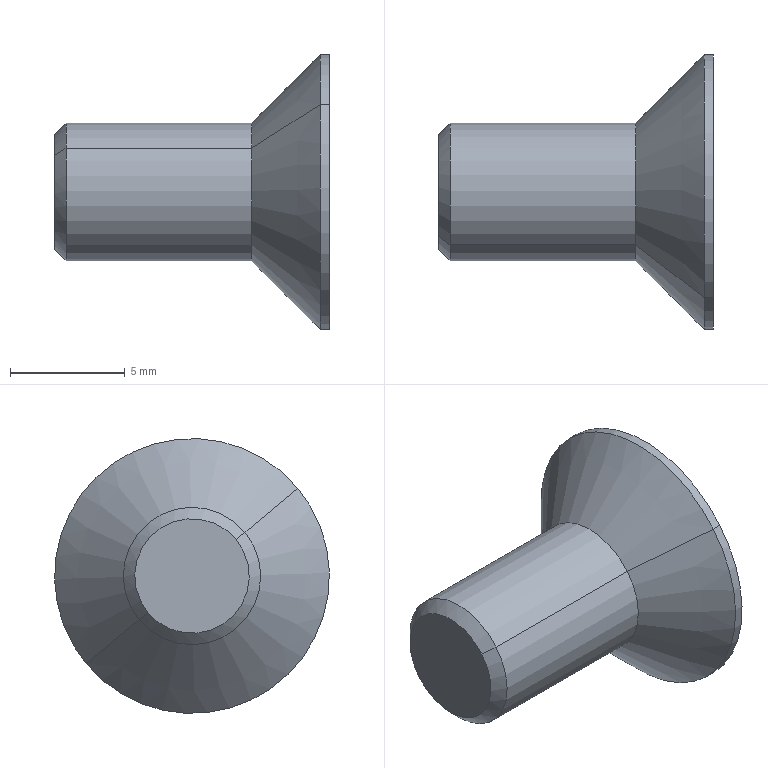Part | STEP file | 平头螺丝(M6) | 1 solid | 17 faces | box 12 x 12 x 12 mm | volume 449.452 mm3 | plane 9 | cone 4 | cylinder 4 | commonest cylinder face diameters 6 x2 12 x2